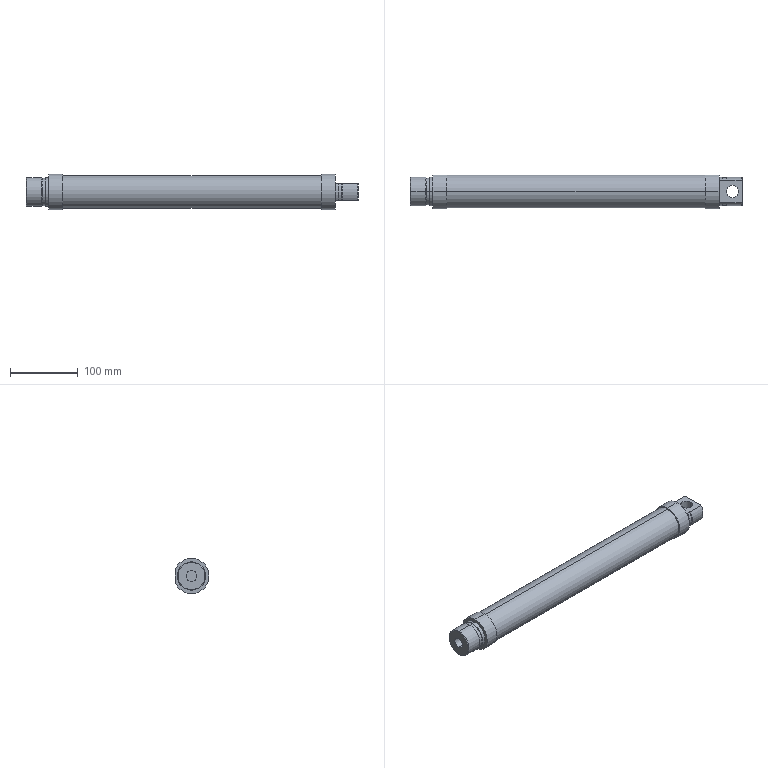Part | STEP file | 1 solid | 59 faces | box 491 x 50.3 x 52 mm | volume 426363 mm3 | cylinder 30 | plane 17 | cone 12 | commonest cylinder face diameters 42 x8 52 x6 11.445 x4 40.159 x4 16 x2 18 x2